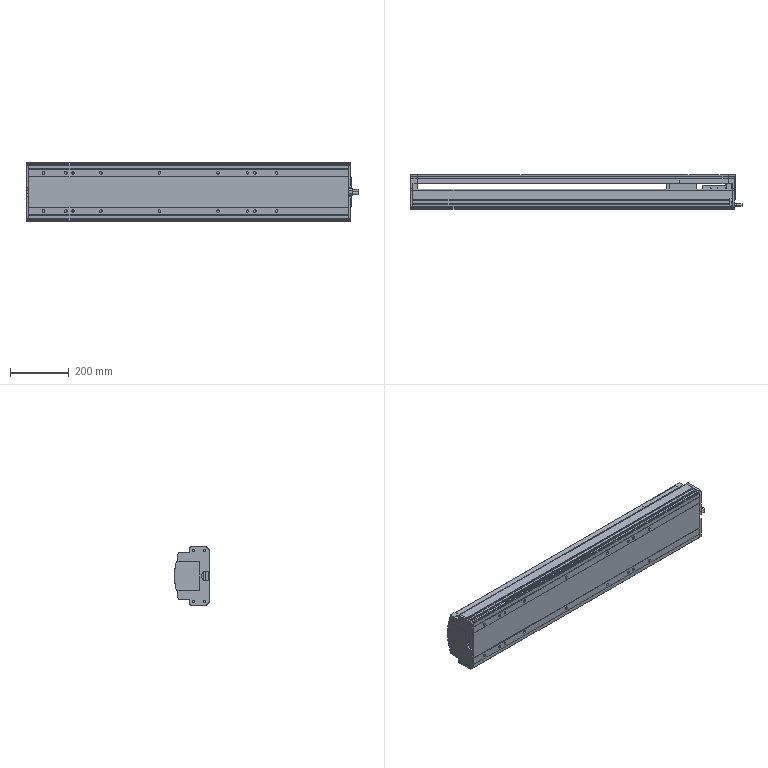Part | STEP file | ISPB-WXM-WA-750-10-650-T4-N-AQ-EB-G3-^-Part-3 | 1 solid | 480 faces | box 1132 x 118.5 x 198 mm | volume 13393000 mm3 | plane 297 | cylinder 183 | commonest cylinder face diameters 9 x36 8 x32 18 x20 7 x16 7.6 x16 6 x12